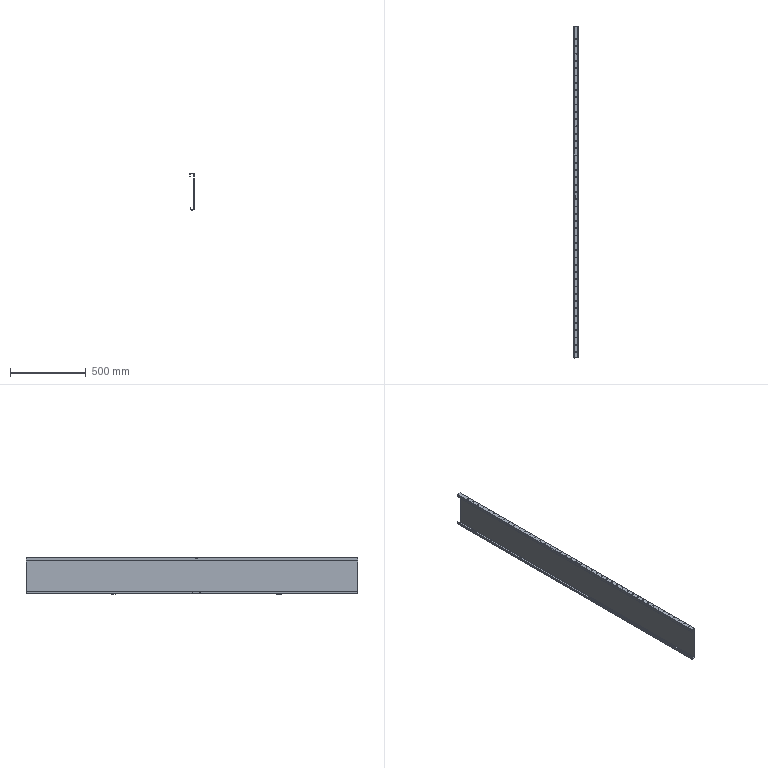Part | NX | features solid 2 | 1 solid | 214 faces | box 29.3 x 2189 x 243.5 mm | volume 1719304 mm3 | cylinder 108 | plane 106 | commonest cylinder face diameters 5.4 x88 0.86 x7 5.86 x7 4 x4 5 x2